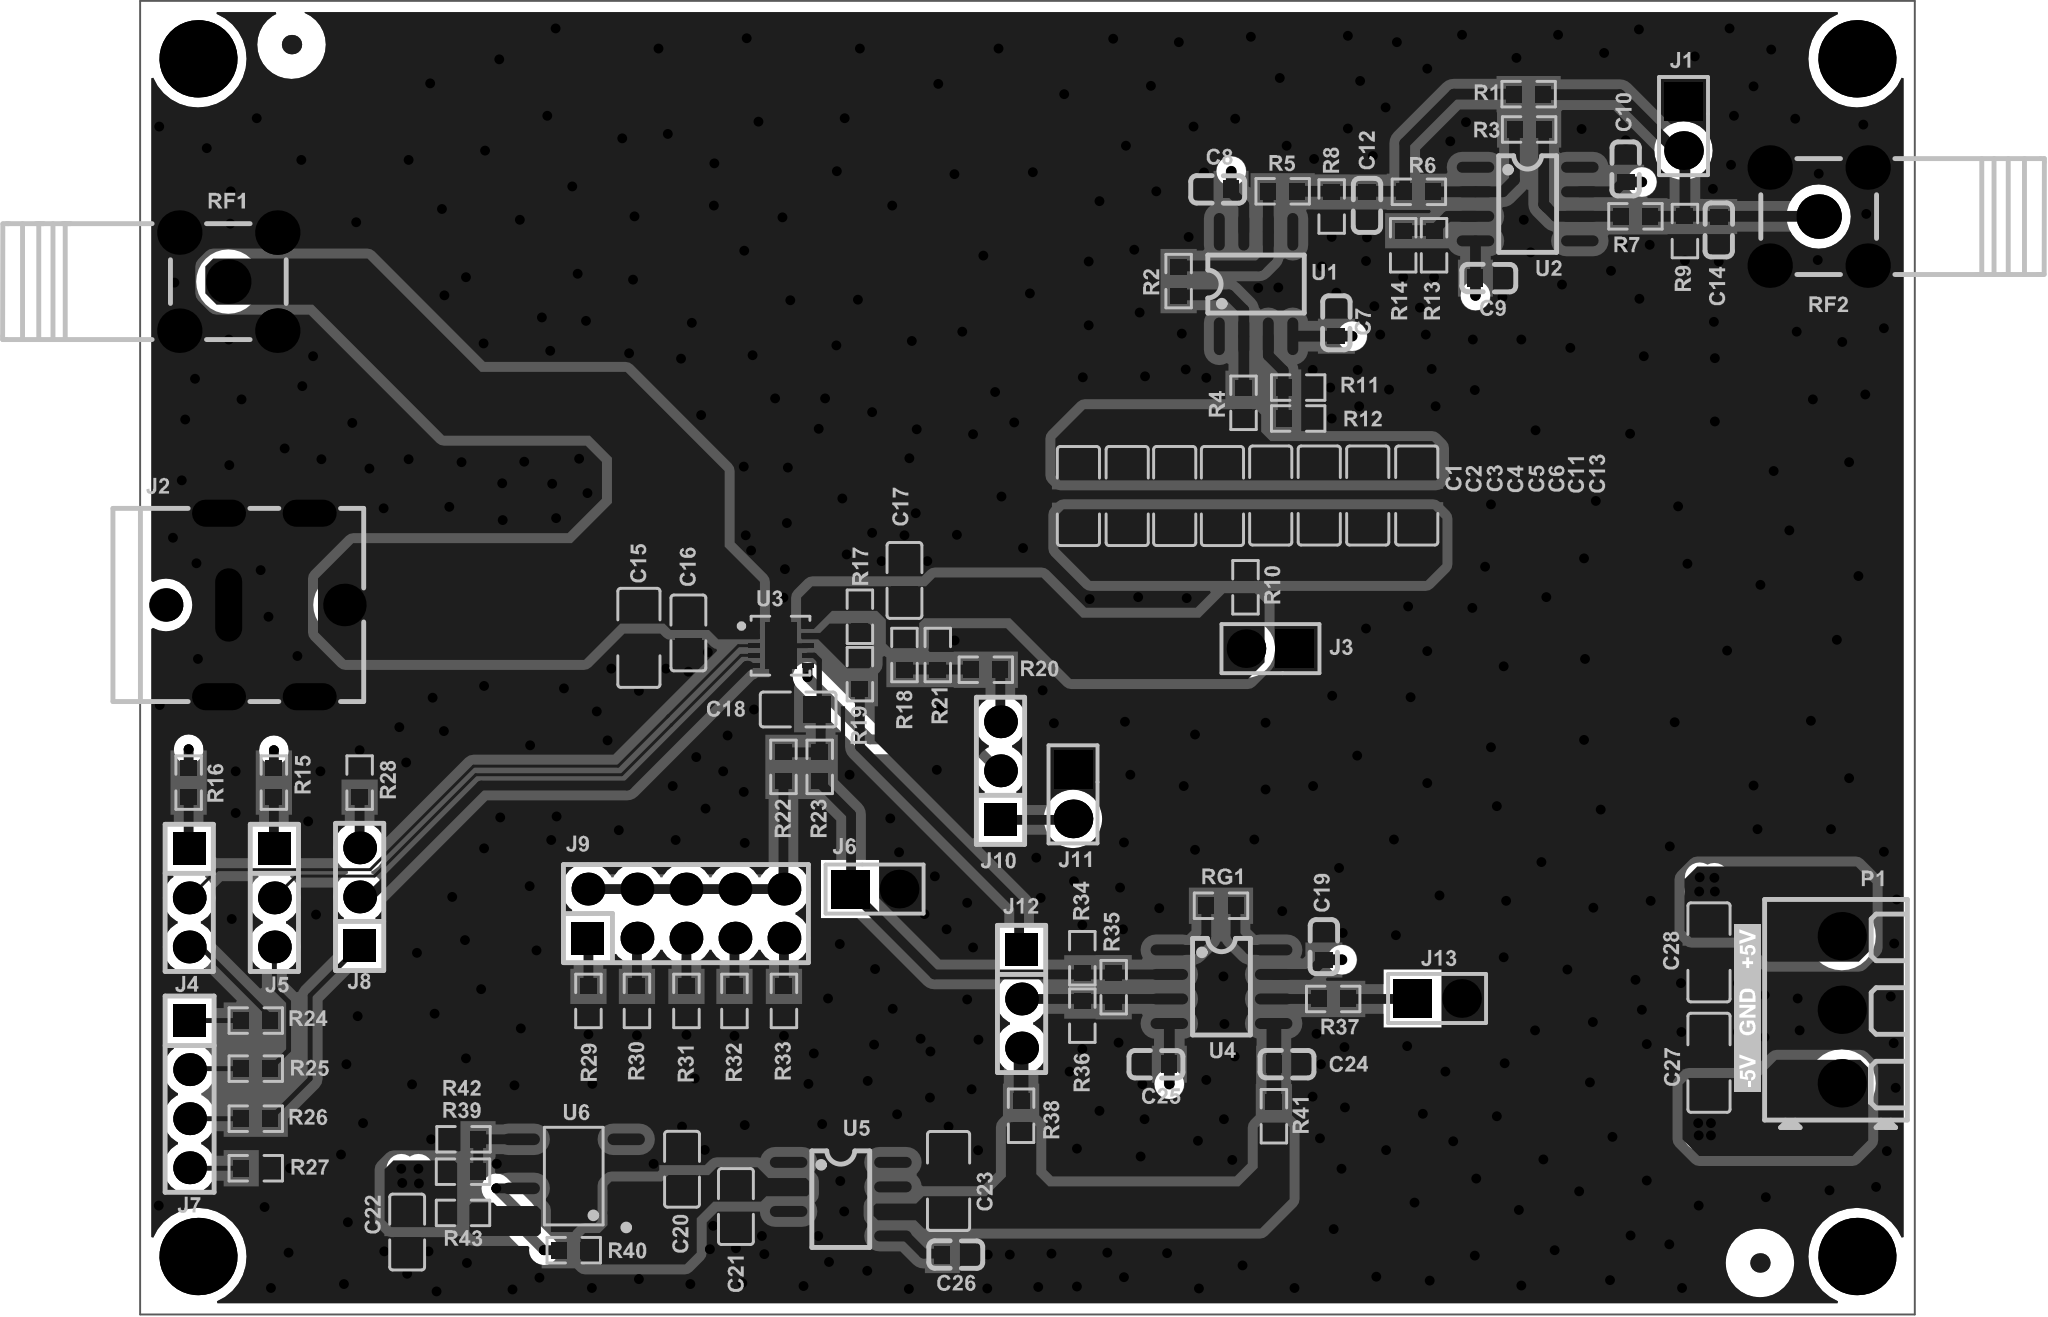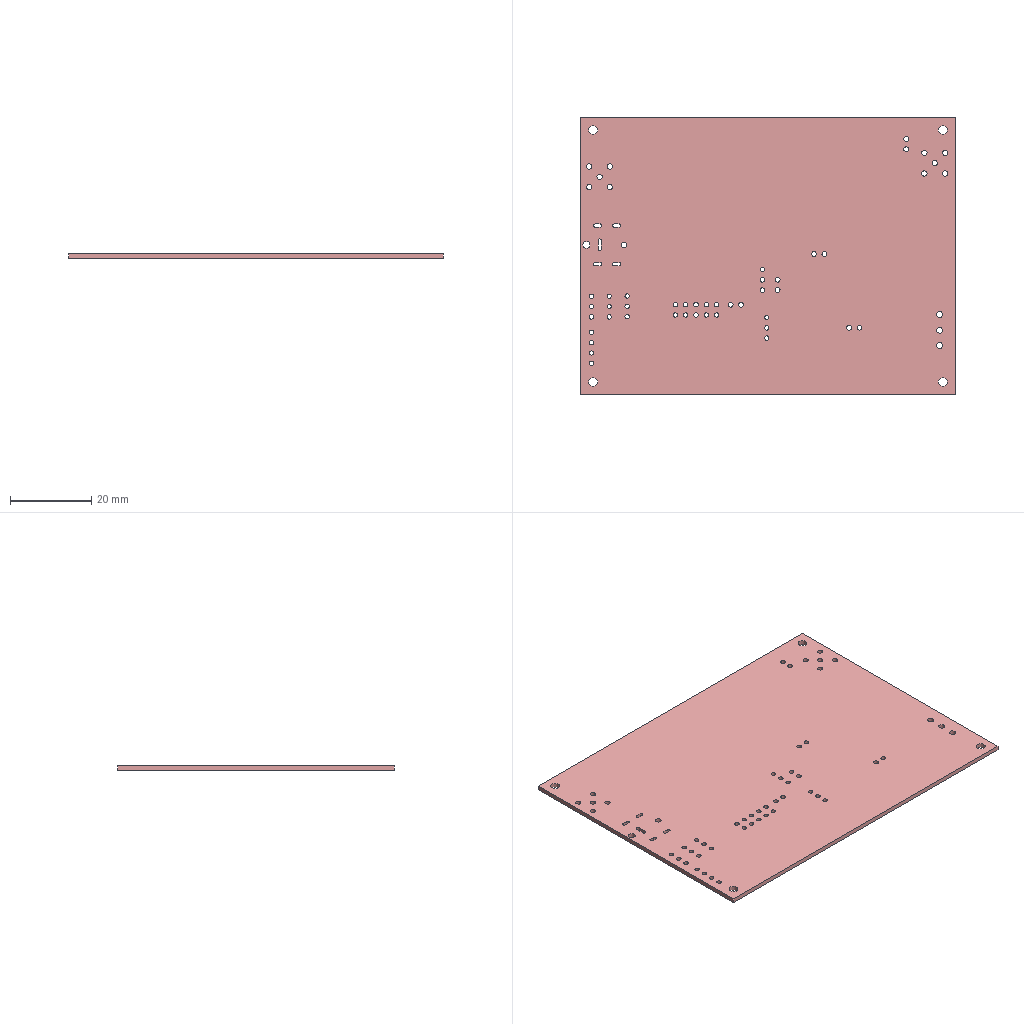Circuit board layout | Altium Designer | box 92 x 68 x 1.1 mm
Layer stack:
# Altium Designer layer stack of  (unit mm; dielectric type: 0 none, 1 core, 2 prepreg, 3 surface material)
index,name,kind,layer,copper_thickness_mm,dielectric_type,dielectric_thickness_mm,dielectric_material,dielectric_constant
0,Top Paste,other,,,,,,
1,Top Overlay,other,,,,,,
2,Top Solder,dielectric,,,3,0.0102,Solder Resist,3.5
3,Top Layer,copper,Top Layer,0.0356,,,,
4,Dielectric1,dielectric,,,1,0.32,FR-4,4.8
5,GND,copper,GND,0.0356,,,,
6,Dielectric2,dielectric,,,2,0.32,FR-4,4.8
7,POWER,copper,POWER,0.0356,,,,
8,Dielectric3,dielectric,,,1,0.32,FR-4,4.8
9,Bottom Layer,copper,Bottom Layer,0.0356,,,,
10,Bottom Solder,dielectric,,,3,0.0102,Solder Resist,3.5
11,Bottom Overlay,other,,,,,,
12,Bottom Paste,other,,,,,,
# drill layer pairs: low layer,high layer
drill_pair,Top Layer,Bottom Layer
Part placement:
Designator,Comment,Layer,Footprint,Center-X(mm),Center-Y(mm),Rotation
C18,4.7u/35V,TopLayer,C0805,34.112,31.318,360
U3,DU3042,TopLayer,WSON-10_L3.0-W3.0-P0.50-BL-EP,33.198,34.62,270
C28,22uF/35V,TopLayer,C1206,81.331,18.745,90
C27,22uF/35V,TopLayer,C1206,81.331,13.03,270
P1,DB125-3.81-3P-GN-S,TopLayer,CONN-TH_3P-P3.81_L7.4-W11.4,88.214,15.773,90
C7,100n/50V,TopLayer,C0603,62.015,51.342,90
C8,100n/50V,TopLayer,C0603,55.855,58.242,180
C9,100n/50V,TopLayer,C0603,69.923,53.646,0
C10,100n/50V,TopLayer,C0603,77.013,59.309,90
C12,100P/50V,TopLayer,C0603,63.599,57.405,270
C14,100P/50V,TopLayer,C0603,81.836,56.135,270
C19,100n/50V,TopLayer,C0603,61.366,19.05,90
C24,100n/50V,TopLayer,C0603,59.461,12.954,360
C25,100n/50V,TopLayer,C0603,52.654,12.954,180
C26,100n/50V,TopLayer,C0603,42.291,3.099,360
J2,HX DC007B-2.5,TopLayer,DC-IN-TH_HX-DC007B-2.5,5.966,36.728,360
R1,NC,TopLayer,R0603,71.981,63.171,180
R2,990R/1%,TopLayer,R0603,53.837,53.494,270
R3,990R/1%,TopLayer,R0603,72.006,61.342,180
R4,100R/1%,TopLayer,R0603,57.201,47.193,90
R5,0R/1%,TopLayer,R0603,59.23,58.142,0
R6,100R/1%,TopLayer,R0603,66.291,58.116,0
R7,0R/1%,TopLayer,R0603,77.518,56.846,0
R8,NC,TopLayer,R0603,61.77,57.354,90
R9,NC,TopLayer,R0603,80.083,56.084,90
R10,0R/1%,TopLayer,R0603,57.302,37.643,270
R11,100R/1%,TopLayer,R0603,60.034,47.982,180
R12,990R/1%,TopLayer,R0603,60.034,46.382,180
R13,100R/1%,TopLayer,R0603,67.079,55.348,90
R14,990R/1%,TopLayer,R0603,65.478,55.348,90
R15,200K/1%,TopLayer,R0603,6.934,27.534,90
R16,1K/1%,TopLayer,R0603,2.515,27.534,90
R17,0R/1%,TopLayer,R0603,37.313,36.119,270
R18,453K/1%,TopLayer,R0603,39.624,34.138,270
R19,0R/1%,TopLayer,R0603,37.313,33.147,270
R20,0R/1%,TopLayer,R0603,43.84,33.376,180
R21,49.9K/1%,TopLayer,R0603,41.351,34.138,90
R22,0R/1%,TopLayer,R0603,33.35,28.346,270
R23,0R/1%,TopLayer,R0603,35.23,28.346,270
R24,0R/1%,TopLayer,R0603,5.994,15.215,180
R25,0R/1%,TopLayer,R0603,5.994,12.725,180
R26,0R/1%,TopLayer,R0603,5.994,10.135,180
R27,0R/1%,TopLayer,R0603,5.994,7.569,180
R28,499R/1%,TopLayer,R0603,11.379,27.534,270
R29,9K/1%,TopLayer,R0603,23.241,16.231,90
R30,18K/1%,TopLayer,R0603,25.756,16.231,90
R31,25K/1%,TopLayer,R0603,28.321,16.231,90
R32,30K/1%,TopLayer,R0603,30.81,16.231,90
R33,50K/1%,TopLayer,R0603,33.376,16.231,90
R34,NC,TopLayer,R0603,48.844,18.44,90
R35,NC,TopLayer,R0603,50.47,16.942,270
R36,NC,TopLayer,R0603,48.844,15.469,270
R37,0R/1%,TopLayer,R0603,61.849,16.332,360
R38,0R/1%,TopLayer,R0603,45.669,10.287,90
R39,100K/1%,TopLayer,R0603,16.739,7.391,180
R40,100K/1%,TopLayer,R0603,22.479,3.327,360
R41,0R/1%,TopLayer,R0603,58.776,10.262,90
R42,100K/1%,TopLayer,R0603,16.764,9.068,360
RG1,505R/1%,TopLayer,R0603,56.032,21.158,180
C1,GRM31CR60J227ME11L,TopLayer,C1206,48.641,42.367,270
C2,GRM31CR60J227ME11L,TopLayer,C1206,51.17,42.368,270
C3,GRM31CR60J227ME11L,TopLayer,C1206,53.633,42.368,270
C4,GRM31CR60J227ME11L,TopLayer,C1206,56.109,42.367,270
C5,22uF/35V,TopLayer,C1206,58.612,42.394,270
C6,22uF/35V,TopLayer,C1206,61.126,42.394,270
C11,22uF/35V,TopLayer,C1206,63.641,42.394,270
C13,22uF/35V,TopLayer,C1206,66.181,42.394,270
C15,22uF/35V,TopLayer,C1206,25.857,35.027,90
C23,22uF/35V,TopLayer,C1206,41.91,6.909,90
C16,4.7u/35V,TopLayer,C0805,28.423,35.281,90
C17,4.7u/35V,TopLayer,C0805,39.624,37.998,270
C20,4.7u/35V,TopLayer,C0805,28.092,7.518,270
C21,4.7u/35V,TopLayer,C0805,30.886,5.588,90
C22,4.7u/35V,TopLayer,C0805,13.843,4.267,90
J7,PZ254V-11-04P_C2691448,TopLayer,HDR-TH_4P-P2.54-V-M,2.565,11.405,270
J4,PZ254V-11-03P_C2937625,TopLayer,HDR-TH_3P-P2.54-V-M,2.545,21.565,270
J5,PZ254V-11-03P_C2937625,TopLayer,HDR-TH_3P-P2.54-V-M,6.96,21.565,270
J8,PZ254V-11-03P_C2937625,TopLayer,HDR-TH_3P-P2.54-V-M,11.379,21.615,90
J10,PZ254V-11-03P_C2937625,TopLayer,HDR-TH_3P-P2.54-V-M,44.602,28.143,90
J1,PZ254V-11-02P,TopLayer,HDR-TH_2P-P2.54-V-M,80.01,61.519,270
J6,PZ254V-11-02P,TopLayer,HDR-TH_2P-P2.54-V-M,38.075,22.022,360
J11,PZ254V-11-02P,TopLayer,HDR-TH_2P-P2.54-V-M,48.362,26.924,270
J12,PZ254V-11-03P_C2937625,TopLayer,HDR-TH_3P-P2.54-V-M,45.695,16.332,270
J13,PZ254V-11-02P,TopLayer,HDR-TH_2P-P2.54-V-M,67.234,16.358,360
J3,PZ254V-11-02P,TopLayer,HDR-TH_2P-P2.54-V-M,58.598,34.468,180
J9,PZ254V-12-10P,TopLayer,HDR-TH_10P-P2.54-V-M-R2-C5-S2.54,28.296,20.752,360
R43,0R/1%,TopLayer,R0603,16.739,5.258,360
RF1,KH-SMA-K513-G,TopLayer,ANT-TH_KH-SMA-K513-G,4.572,53.467,360
RF2,KH-SMA-K513-G,TopLayer,ANT-TH_KH-SMA-K513-G,87.018,56.834,180
U1,OPA211IDR,TopLayer,SOIC-8_L5.0-W4.0-P1.27-LS6.0-BL,57.85,53.341,360
U2,OPA211IDR,TopLayer,SOIC-8_L5.0-W4.0-P1.27-LS6.0-BL,71.93,57.481,270
U4,INA828IDR,TopLayer,SOIC-8_L5.0-W4.0-P1.27-LS6.0-BL,56.058,16.967,270
U5,REF5025AIDR,TopLayer,SOIC-8_L5.0-W4.0-P1.27-LS6.0-BL,36.322,5.969,270
U6,ADP7104ARDZ-5.0-R7,TopLayer,SOIC-8_L4.9-W3.9-P1.27-LS6.0-BL-EP,22.479,7.163,90
Pad and via stacks:
# Altium Designer via and pad stacks of  (unit mm). Each distinct definition once, with the count of objects using it.
# via: kind,start_layer,end_layer,hole_mm,diameter_mm,mode(0 simple;1 top-mid-bottom;2 full stack),diameter_per_layer,count,example_net
# pad: kind,layer,hole_mm,hole_type(0 round;1 square;2 slot),plating,top_size,top_shape(1 round;2 rect;3 octagon;9 rounded rect),mid_size,bottom_size,mode,footprint,size_per_layer,count,example
pad,Top Layer,0,0,plated,0.8065x0.864,2,0.8065x0.864,0.8065x0.864,0,R0603,,88,R40.2
pad,Top Layer,0,0,plated,1.41x1.35,2,1.41x1.35,1.41x1.35,0,C0805,,12,C18.2
pad,Top Layer,0,0,plated,1.485x1.728,2,1.485x1.728,1.485x1.728,0,C1206,,24,C15.2
pad,Top Layer,0,0,plated,0.25x0.6,2,0.25x0.6,0.25x0.6,0,WSON-10_L3.0-W3.0-P0.50-BL-EP,,10,U3.10
pad,Top Layer,0,0,plated,2.4x1.65,2,2.4x1.65,2.4x1.65,0,WSON-10_L3.0-W3.0-P0.50-BL-EP,,1,U3.11
pad,Top Layer,0,0,plated,1x1,1,1x1,1x1,0,,,2,MARK
pad,Top Layer,0,0,plated,0.8x0.9,2,0.8x0.9,0.8x0.9,0,C0603,,20,C10.2
pad,Top Layer,0,0,plated,0.602x1.941,1,0.602x1.941,0.602x1.941,0,SOIC-8_L4.9-W3.9-P1.27-LS6.0-BL-EP,,8,U6.1
pad,Top Layer,0,0,plated,3.098x2.41,2,3.098x2.41,3.098x2.41,0,SOIC-8_L4.9-W3.9-P1.27-LS6.0-BL-EP,,1,U6.9
pad,Top Layer,0,0,plated,0.5684x1.95,1,0.5684x1.95,0.5684x1.95,0,SOIC-8_L5.0-W4.0-P1.27-LS6.0-BL,,32,U1.1
pad,Multi-Layer,1.5,0,plated,2.5x2.5,1,2.5x2.5,2.5x2.5,0,CONN-TH_3P-P3.81_L7.4-W11.4,,3,P1.3
pad,Multi-Layer,2.2,0,plated,4x4,1,4x4,4x4,0,,,4,6
pad,Multi-Layer,1.3,0,plated,2.3x2.3,1,2.3x2.3,2.3x2.3,0,ANT-TH_KH-SMA-K513-G,,10,RF1.1
pad,Multi-Layer,1.1,0,plated,1.7x1.7,2,1.7x1.7,1.7x1.7,0,HDR-TH_10P-P2.54-V-M-R2-C5-S2.54,,1,J9.1
pad,Multi-Layer,1.1,0,plated,1.7x1.7,1,1.7x1.7,1.7x1.7,0,HDR-TH_10P-P2.54-V-M-R2-C5-S2.54,,9,J9.2
pad,Multi-Layer,1.2,0,plated,2x2,2,2x2,2x2,0,HDR-TH_2P-P2.54-V-M,,5,J1.1
pad,Multi-Layer,1.2,0,plated,2x2,1,2x2,2x2,0,HDR-TH_2P-P2.54-V-M,,5,J1.2
pad,Multi-Layer,1.1,0,plated,1.7x1.7,2,1.7x1.7,1.7x1.7,0,HDR-TH_3P-P2.54-V-M,,5,J4.1
pad,Multi-Layer,1.1,0,plated,1.7x1.7,1,1.7x1.7,1.7x1.7,0,HDR-TH_3P-P2.54-V-M,,10,J4.2
pad,Multi-Layer,1.1,0,plated,1.7x1.7,2,1.7x1.7,1.7x1.7,0,HDR-TH_4P-P2.54-V-M,,1,J7.1
pad,Multi-Layer,1.1,0,plated,1.7x1.7,1,1.7x1.7,1.7x1.7,0,HDR-TH_4P-P2.54-V-M,,3,J7.2
pad,Multi-Layer,0.8,2,plated,1.4x2.8,1,1.4x2.8,1.4x2.8,0,DC-IN-TH_HX-DC007B-2.5,,4,J2.3
pad,Multi-Layer,0.8,2,plated,1.4x3.8,1,1.4x3.8,1.4x3.8,0,DC-IN-TH_HX-DC007B-2.5,,1,J2.2
pad,Multi-Layer,1.4,0,plated,2.2x2.2,1,2.2x2.2,2.2x2.2,0,DC-IN-TH_HX-DC007B-2.5,,1,J2.1
pad,Multi-Layer,1.7,0,unplated,1.7x1.7,1,1.7x1.7,1.7x1.7,0,DC-IN-TH_HX-DC007B-2.5,,1,J2.0
pad,Bottom Layer,0,0,plated,1x1,1,1x1,1x1,0,,,2,MARK
via,Top Layer,Bottom Layer,0.3048,0.508,0,,522,GND
Copper pours:
name,layer,net,type(0 solid;1 hatched;2 none)
Bottom Layer-No Net,Top Layer,VIN,0
Bottom Layer-No Net,Top Layer,REF_5V,0
Bottom Layer-No Net,Top Layer,NetC1_1,0
Bottom Layer-No Net,Top Layer,NetC1_2,0
Bottom Layer-No Net,Top Layer,NetC17_2,0
Bottom Layer-No Net,Top Layer,NetR17_2,0
Bottom Layer-No Net,Top Layer,GND,0
Bottom Layer-No Net,Top Layer,-5V,0
Bottom Layer-No Net,Top Layer,REF_2.5V,0
Bottom Layer-No Net,Top Layer,NetR43_2,0
Bottom Layer-No Net,Top Layer,VIN,0
Bottom Layer-No Net,Top Layer,+5V,0
Bottom Layer-No Net,Bottom Layer,GND,0
Design rules, without the lines most boards share:
# Altium Designer design rules of  (exported by Altium Designer, unit mm)
# columns: name | kind | enabled | priority | scope1 | scope2 | descriptor | typed fields (field=value)
Clearance_3 | 0 | enabled | 1 | HASPAD('FREE-MARK') | All | Clearance Constraint (Gap=50mil) (HASPAD('FREE-MARK')),(All) | gap=1.27
Clearance_2 | 0 | enabled | 2 | INPOLYGON | All | Clearance Constraint (Gap=6mil) (INPOLYGON),(All) | gap=0.1524
Clearance | 0 | enabled | 3 | All | All | Clearance Constraint (Gap=6mil) (All),(All) | gap=0.1524
PlaneConnect | 6 | enabled | 1 | All | All | Power Plane Connect Rule(Direct Connect )(Expansion=20mil) (Conductor Width=10mil) (Air Gap=10mil) (Entries=4) (All) | relief_conductor_width=0.254 relief_entries=4 relief_expansion=0.508
PlaneClearance | 12 | enabled | 1 | All | All | Power Plane Clearance (Clearance =10mil) (All) | clearance=0.254
PolygonConnect | 20 | enabled | 1 | All | All | Polygon Connect Rule(Direct Connect )(Conductor Width=10mil) (Relief Angle=90 Angle) (Entries=4) (Air Gap Width=10mil) (All),(All) | connect_style(0=relief,1=direct,2=none)=1 relief_conductor_width=0.254 relief_entries=4
Width | 2 | enabled | 1 | All | All | Width Constraint (Min=6mil) (Max=40mil) (Preferred=6mil) (All) |
RoutingVias | 11 | enabled | 1 | All | All | Routing Via (MinHoleWidth=12mil) (MaxHoleWidth=12mil) (PreferredHoleWidth=12mil) (MinWidth=20mil) (MaxWidth=20mil) (PreferedWidth=20mil) (All) | via_min_hole=0.3048 via_max_hole=0.3048 via_preferred_diameter=0.508 via_preferred_hole=0.3048
SolderMaskExpansion | 13 | enabled | 1 | All | All | Solder Mask Expansion (Expansion =4mil) (All) | expansion=0.1016
HoleSize | 42 | enabled | 1 | All | All | Hole Size Constraint (Min=1mil) (Max=500mil) (All) |
DiffPairsRouting | 51 | enabled | 1 | All | All | Differential Pairs Uncoupled Length using the Gap Constraints (Min=6mil) (Max=6mil) (Prefered=6mil)  and Width Constraints (Min=15mil) (Max=15mil) (Prefered=15mil) (All) |
HoleToHoleClearance | 52 | enabled | 1 | All | All | Hole To Hole Clearance (Gap=0mil) (All),(All) | gap=0
MinimumSolderMaskSliver | 53 | enabled | 1 | All | All | Minimum Solder Mask Sliver (Gap=0mil) (All),(All) |
SilkscreenOverComponentPads | 54 | enabled | 1 | IsPad | All | Silk To Solder Mask (Clearance=0mil) (IsPad),(All) |
SilkToSilkClearance | 55 | enabled | 1 | All | All | Silk to Silk (Clearance=0mil) (All),(All) |
Classes set for this board:
# Altium Designer classes of  (member kind: 0 net, 1 component, 2 from-to, 3 pad, 4 layer, 5 differential pair, 6 design channel, 7 polygon, 8 structure, 9 xSignal)
# columns: class name | member kind | superclass | members
Sheet1 | 1 | no | C1; C2; C3; C4; C5; C6; C7; C8; C9; C10; C11; C12; C13; C14; C15; C16; C17; C18; C19; C20; C21; C22; C23; C24; C25; C26; J1; J2; J3; J4; J5; J6; J7; J8; J9; J10; J11; J12; J13; R1; R2; R3; R4; R5; R6; R7; R8; R9; R10; R11; R12; R13; R14; R15; R16; R17; R18; R19; R20; R21; R22; R23; R24; R25; R26; R27; R28; R29; R30; R31; R32; R33; R34; R35; R36; R37; R38; R39; R40; R41; R42; RF1; RG1; U1; U2; U3; U4; U5; U6; C1; C2; C3; C4; C5; C6; C11; C13; C15; C23; C16; C17; C18; C20; C21; C22; J7; J4; J5; J8; J10; J1; J6; J11; J12; J13; J3; J9; R43; RF1; RF2; U1; U2; U4; U5; U6; U3; P1; U3; C27; C28; U3; U3; U3;